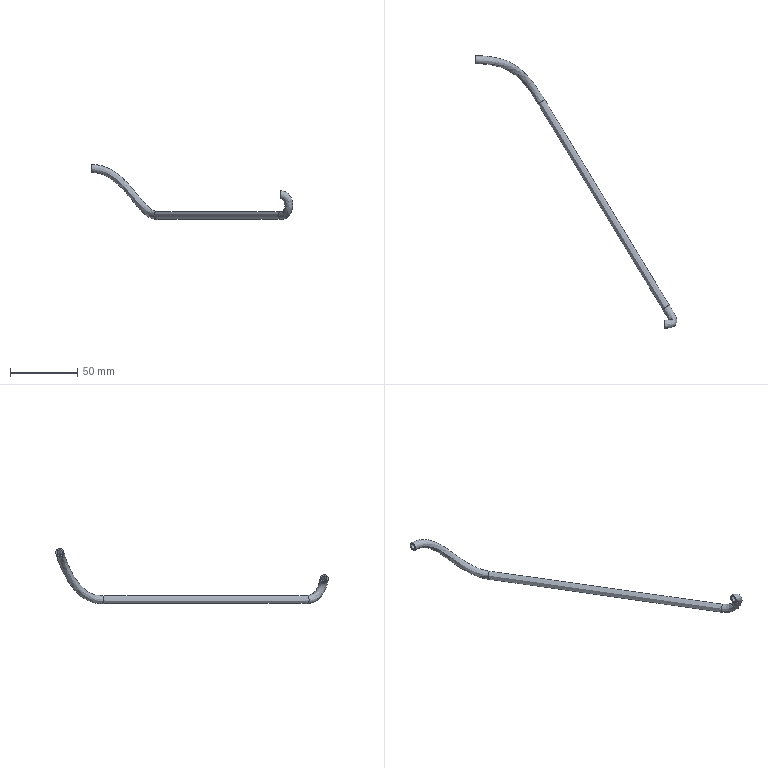Part | NX | features solid 2 | 1 solid | 8 faces | box 149.405 x 202 x 41.009 mm | volume 4361 mm3 | spline 6 | plane 2